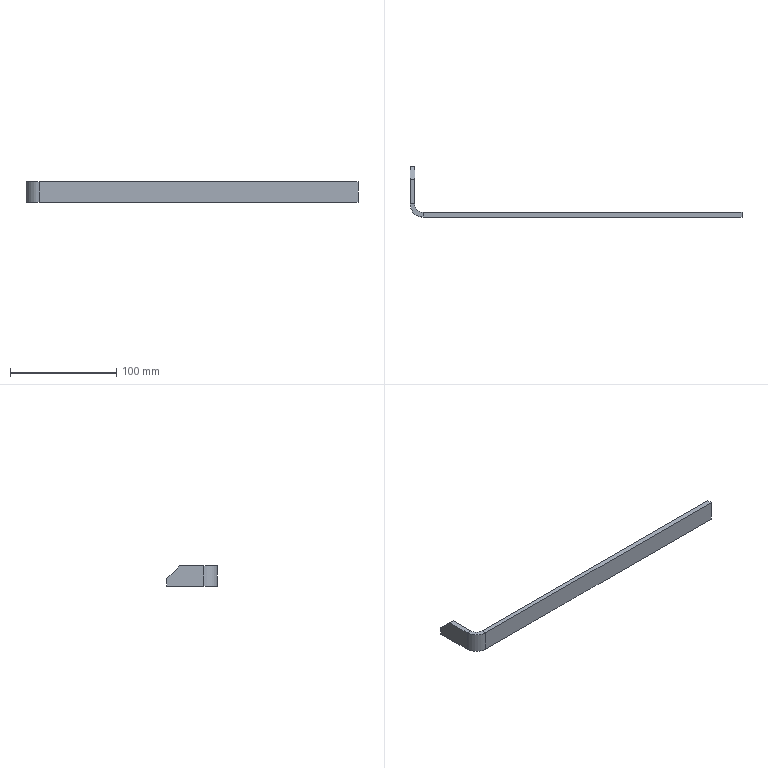Part | SolidWorks | features Chamfer 1, FlatPattern 1, SMBaseFlange 1, SheetMetal 1 | 1 solid | 15 faces | box 313 x 47.5 x 19 mm | volume 29738 mm3 | plane 13 | cylinder 2 | commonest cylinder face diameters 16 x1 25 x1
STEP:
#1=CARTESIAN_POINT('',(0.,-35.,9.5));
#2=VERTEX_POINT('',#1);
#3=CARTESIAN_POINT('',(4.5,-35.,9.5));
#4=VERTEX_POINT('',#3);
#5=CARTESIAN_POINT('',(0.,-35.,9.5));
#6=DIRECTION('',(1.,0.,0.));
#7=VECTOR('',#6,1000.);
#8=LINE('',#5,#7);
#9=EDGE_CURVE('',#2,#4,#8,.T.);
#10=ORIENTED_EDGE('',*,*,#9,.F.);
#11=CARTESIAN_POINT('',(12.5,-47.5,9.5));
#12=VERTEX_POINT('',#11);
#13=CARTESIAN_POINT('',(12.5,-35.,9.5));
#14=DIRECTION('',(0.,0.,1.));
#15=DIRECTION('',(-1.,0.,0.));
#16=AXIS2_PLACEMENT_3D('',#13,#14,#15);
#17=CIRCLE('',#16,12.5);
#18=EDGE_CURVE('',#2,#12,#17,.T.);
#19=ORIENTED_EDGE('',*,*,#18,.T.);
#20=CARTESIAN_POINT('',(12.5,-43.,9.5));
#21=VERTEX_POINT('',#20);
#22=CARTESIAN_POINT('',(12.5,-43.,9.5));
#23=DIRECTION('',(0.,-1.,0.));
#24=VECTOR('',#23,1000.);
#25=LINE('',#22,#24);
#26=EDGE_CURVE('',#21,#12,#25,.T.);
#27=ORIENTED_EDGE('',*,*,#26,.F.);
#28=CARTESIAN_POINT('',(12.5,-35.,9.5));
#29=DIRECTION('',(0.,0.,1.));
#30=DIRECTION('',(1.,0.,0.));
#31=AXIS2_PLACEMENT_3D('',#28,#29,#30);
#32=CIRCLE('',#31,8.);
#33=EDGE_CURVE('',#4,#21,#32,.T.);
#34=ORIENTED_EDGE('',*,*,#33,.F.);
#35=EDGE_LOOP('',(#10,#19,#27,#34));
#36=FACE_OUTER_BOUND('',#35,.T.);
#37=CARTESIAN_POINT('',(0.,-35.,9.5));
#38=DIRECTION('',(0.,0.,1.));
#39=DIRECTION('',(1.,0.,0.));
#40=AXIS2_PLACEMENT_3D('',#37,#38,#39);
#41=PLANE('',#40);
#42=ADVANCED_FACE('',(#36),#41,.T.);
#43=CARTESIAN_POINT('',(4.5,-12.,9.5));
#44=VERTEX_POINT('',#43);
#45=CARTESIAN_POINT('',(4.5,0.,9.5));
#46=DIRECTION('',(0.,-1.,0.));
#47=VECTOR('',#46,1000.);
#48=LINE('',#45,#47);
#49=EDGE_CURVE('',#44,#4,#48,.T.);
#50=ORIENTED_EDGE('',*,*,#49,.F.);
#51=CARTESIAN_POINT('',(0.,-12.,9.5));
#52=VERTEX_POINT('',#51);
#53=CARTESIAN_POINT('',(12.5,-12.,9.5));
#54=DIRECTION('',(-1.,0.,0.));
#55=VECTOR('',#54,1000.);
#56=LINE('',#53,#55);
#57=EDGE_CURVE('',#44,#52,#56,.T.);
#58=ORIENTED_EDGE('',*,*,#57,.T.);
#59=CARTESIAN_POINT('',(0.,0.,9.5));
#60=DIRECTION('',(0.,-1.,0.));
#61=VECTOR('',#60,1000.);
#62=LINE('',#59,#61);
#63=EDGE_CURVE('',#52,#2,#62,.T.);
#64=ORIENTED_EDGE('',*,*,#63,.T.);
#65=ORIENTED_EDGE('',*,*,#9,.T.);
#66=EDGE_LOOP('',(#50,#58,#64,#65));
#67=FACE_OUTER_BOUND('',#66,.T.);
#68=CARTESIAN_POINT('',(12.5,-43.,9.5));
#69=DIRECTION('',(0.,0.,1.));
#70=DIRECTION('',(1.,0.,0.));
#71=AXIS2_PLACEMENT_3D('',#68,#69,#70);
#72=PLANE('',#71);
#73=ADVANCED_FACE('',(#67),#72,.T.);
#74=CARTESIAN_POINT('',(12.5,-47.5,-9.5));
#75=VERTEX_POINT('',#74);
#76=CARTESIAN_POINT('',(12.5,-43.,-9.5));
#77=VERTEX_POINT('',#76);
#78=CARTESIAN_POINT('',(12.5,-47.5,-9.5));
#79=DIRECTION('',(0.,1.,0.));
#80=VECTOR('',#79,1000.);
#81=LINE('',#78,#80);
#82=EDGE_CURVE('',#75,#77,#81,.T.);
#83=ORIENTED_EDGE('',*,*,#82,.F.);
#84=CARTESIAN_POINT('',(0.,-35.,-9.5));
#85=VERTEX_POINT('',#84);
#86=CARTESIAN_POINT('',(12.5,-35.,-9.5));
#87=DIRECTION('',(0.,0.,1.));
#88=DIRECTION('',(-1.,0.,0.));
#89=AXIS2_PLACEMENT_3D('',#86,#87,#88);
#90=CIRCLE('',#89,12.5);
#91=EDGE_CURVE('',#85,#75,#90,.T.);
#92=ORIENTED_EDGE('',*,*,#91,.F.);
#93=CARTESIAN_POINT('',(4.5,-35.,-9.5));
#94=VERTEX_POINT('',#93);
#95=CARTESIAN_POINT('',(4.5,-35.,-9.5));
#96=DIRECTION('',(-1.,0.,0.));
#97=VECTOR('',#96,1000.);
#98=LINE('',#95,#97);
#99=EDGE_CURVE('',#94,#85,#98,.T.);
#100=ORIENTED_EDGE('',*,*,#99,.F.);
#101=CARTESIAN_POINT('',(12.5,-35.,-9.5));
#102=DIRECTION('',(0.,0.,1.));
#103=DIRECTION('',(1.,0.,0.));
#104=AXIS2_PLACEMENT_3D('',#101,#102,#103);
#105=CIRCLE('',#104,8.);
#106=EDGE_CURVE('',#94,#77,#105,.T.);
#107=ORIENTED_EDGE('',*,*,#106,.T.);
#108=EDGE_LOOP('',(#83,#92,#100,#107));
#109=FACE_OUTER_BOUND('',#108,.T.);
#110=CARTESIAN_POINT('',(12.5,-47.5,-9.5));
#111=DIRECTION('',(0.,0.,-1.));
#112=DIRECTION('',(-1.,0.,0.));
#113=AXIS2_PLACEMENT_3D('',#110,#111,#112);
#114=PLANE('',#113);
#115=ADVANCED_FACE('',(#109),#114,.T.);
#116=CARTESIAN_POINT('',(313.,-47.5,-9.5));
#117=VERTEX_POINT('',#116);
#118=CARTESIAN_POINT('',(0.,-47.5,-9.5));
#119=DIRECTION('',(1.,0.,0.));
#120=VECTOR('',#119,1000.);
#121=LINE('',#118,#120);
#122=EDGE_CURVE('',#75,#117,#121,.T.);
#123=ORIENTED_EDGE('',*,*,#122,.F.);
#124=ORIENTED_EDGE('',*,*,#82,.T.);
#125=CARTESIAN_POINT('',(313.,-43.,-9.5));
#126=VERTEX_POINT('',#125);
#127=CARTESIAN_POINT('',(0.,-43.,-9.5));
#128=DIRECTION('',(1.,0.,0.));
#129=VECTOR('',#128,1000.);
#130=LINE('',#127,#129);
#131=EDGE_CURVE('',#77,#126,#130,.T.);
#132=ORIENTED_EDGE('',*,*,#131,.T.);
#133=CARTESIAN_POINT('',(313.,-43.,-9.5));
#134=DIRECTION('',(0.,-1.,0.));
#135=VECTOR('',#134,1000.);
#136=LINE('',#133,#135);
#137=EDGE_CURVE('',#126,#117,#136,.T.);
#138=ORIENTED_EDGE('',*,*,#137,.T.);
#139=EDGE_LOOP('',(#123,#124,#132,#138));
#140=FACE_OUTER_BOUND('',#139,.T.);
#141=CARTESIAN_POINT('',(4.5,-35.,-9.5));
#142=DIRECTION('',(0.,0.,-1.));
#143=DIRECTION('',(-1.,0.,0.));
#144=AXIS2_PLACEMENT_3D('',#141,#142,#143);
#145=PLANE('',#144);
#146=ADVANCED_FACE('',(#140),#145,.T.);
#147=ORIENTED_EDGE('',*,*,#122,.T.);
#148=CARTESIAN_POINT('',(313.,-47.5,9.5));
#149=VERTEX_POINT('',#148);
#150=CARTESIAN_POINT('',(313.,-47.5,9.5));
#151=DIRECTION('',(0.,0.,-1.));
#152=VECTOR('',#151,1000.);
#153=LINE('',#150,#152);
#154=EDGE_CURVE('',#149,#117,#153,.T.);
#155=ORIENTED_EDGE('',*,*,#154,.F.);
#156=CARTESIAN_POINT('',(0.,-47.5,9.5));
#157=DIRECTION('',(1.,0.,0.));
#158=VECTOR('',#157,1000.);
#159=LINE('',#156,#158);
#160=EDGE_CURVE('',#12,#149,#159,.T.);
#161=ORIENTED_EDGE('',*,*,#160,.F.);
#162=CARTESIAN_POINT('',(12.5,-47.5,9.5));
#163=DIRECTION('',(0.,0.,-1.));
#164=VECTOR('',#163,1000.);
#165=LINE('',#162,#164);
#166=EDGE_CURVE('',#12,#75,#165,.T.);
#167=ORIENTED_EDGE('',*,*,#166,.T.);
#168=EDGE_LOOP('',(#147,#155,#161,#167));
#169=FACE_OUTER_BOUND('',#168,.T.);
#170=CARTESIAN_POINT('',(0.,-47.5,9.5));
#171=DIRECTION('',(0.,1.,0.));
#172=DIRECTION('',(0.,0.,1.));
#173=AXIS2_PLACEMENT_3D('',#170,#171,#172);
#174=PLANE('',#173);
#175=ADVANCED_FACE('',(#169),#174,.F.);
#176=ORIENTED_EDGE('',*,*,#137,.F.);
#177=CARTESIAN_POINT('',(313.,-43.,9.5));
#178=VERTEX_POINT('',#177);
#179=CARTESIAN_POINT('',(313.,-43.,9.5));
#180=DIRECTION('',(0.,0.,-1.));
#181=VECTOR('',#180,1000.);
#182=LINE('',#179,#181);
#183=EDGE_CURVE('',#178,#126,#182,.T.);
#184=ORIENTED_EDGE('',*,*,#183,.F.);
#185=CARTESIAN_POINT('',(313.,-43.,9.5));
#186=DIRECTION('',(0.,-1.,0.));
#187=VECTOR('',#186,1000.);
#188=LINE('',#185,#187);
#189=EDGE_CURVE('',#178,#149,#188,.T.);
#190=ORIENTED_EDGE('',*,*,#189,.T.);
#191=ORIENTED_EDGE('',*,*,#154,.T.);
#192=EDGE_LOOP('',(#176,#184,#190,#191));
#193=FACE_OUTER_BOUND('',#192,.T.);
#194=CARTESIAN_POINT('',(313.,-43.,9.5));
#195=DIRECTION('',(1.,0.,0.));
#196=DIRECTION('',(0.,0.,-1.));
#197=AXIS2_PLACEMENT_3D('',#194,#195,#196);
#198=PLANE('',#197);
#199=ADVANCED_FACE('',(#193),#198,.T.);
#200=ORIENTED_EDGE('',*,*,#131,.F.);
#201=CARTESIAN_POINT('',(12.5,-43.,9.5));
#202=DIRECTION('',(0.,0.,-1.));
#203=VECTOR('',#202,1000.);
#204=LINE('',#201,#203);
#205=EDGE_CURVE('',#21,#77,#204,.T.);
#206=ORIENTED_EDGE('',*,*,#205,.F.);
#207=CARTESIAN_POINT('',(0.,-43.,9.5));
#208=DIRECTION('',(1.,0.,0.));
#209=VECTOR('',#208,1000.);
#210=LINE('',#207,#209);
#211=EDGE_CURVE('',#21,#178,#210,.T.);
#212=ORIENTED_EDGE('',*,*,#211,.T.);
#213=ORIENTED_EDGE('',*,*,#183,.T.);
#214=EDGE_LOOP('',(#200,#206,#212,#213));
#215=FACE_OUTER_BOUND('',#214,.T.);
#216=CARTESIAN_POINT('',(0.,-43.,9.5));
#217=DIRECTION('',(0.,1.,0.));
#218=DIRECTION('',(0.,0.,1.));
#219=AXIS2_PLACEMENT_3D('',#216,#217,#218);
#220=PLANE('',#219);
#221=ADVANCED_FACE('',(#215),#220,.T.);
#222=ORIENTED_EDGE('',*,*,#106,.F.);
#223=CARTESIAN_POINT('',(4.5,-35.,9.5));
#224=DIRECTION('',(0.,0.,-1.));
#225=VECTOR('',#224,1000.);
#226=LINE('',#223,#225);
#227=EDGE_CURVE('',#4,#94,#226,.T.);
#228=ORIENTED_EDGE('',*,*,#227,.F.);
#229=ORIENTED_EDGE('',*,*,#33,.T.);
#230=ORIENTED_EDGE('',*,*,#205,.T.);
#231=EDGE_LOOP('',(#222,#228,#229,#230));
#232=FACE_OUTER_BOUND('',#231,.T.);
#233=CARTESIAN_POINT('',(12.5,-35.,9.5));
#234=DIRECTION('',(0.,0.,-1.));
#235=DIRECTION('',(-1.,0.,0.));
#236=AXIS2_PLACEMENT_3D('',#233,#234,#235);
#237=CYLINDRICAL_SURFACE('',#236,8.);
#238=ADVANCED_FACE('',(#232),#237,.F.);
#239=CARTESIAN_POINT('',(4.5,0.,-2.5));
#240=VERTEX_POINT('',#239);
#241=CARTESIAN_POINT('',(4.5,0.,-9.5));
#242=VERTEX_POINT('',#241);
#243=CARTESIAN_POINT('',(4.5,0.,9.5));
#244=DIRECTION('',(0.,0.,-1.));
#245=VECTOR('',#244,1000.);
#246=LINE('',#243,#245);
#247=EDGE_CURVE('',#240,#242,#246,.T.);
#248=ORIENTED_EDGE('',*,*,#247,.F.);
#249=CARTESIAN_POINT('',(4.5,-6.,3.5));
#250=DIRECTION('',(0.,-0.7071,0.7071));
#251=VECTOR('',#250,1000.);
#252=LINE('',#249,#251);
#253=EDGE_CURVE('',#240,#44,#252,.T.);
#254=ORIENTED_EDGE('',*,*,#253,.T.);
#255=ORIENTED_EDGE('',*,*,#49,.T.);
#256=ORIENTED_EDGE('',*,*,#227,.T.);
#257=CARTESIAN_POINT('',(4.5,0.,-9.5));
#258=DIRECTION('',(0.,-1.,0.));
#259=VECTOR('',#258,1000.);
#260=LINE('',#257,#259);
#261=EDGE_CURVE('',#242,#94,#260,.T.);
#262=ORIENTED_EDGE('',*,*,#261,.F.);
#263=EDGE_LOOP('',(#248,#254,#255,#256,#262));
#264=FACE_OUTER_BOUND('',#263,.T.);
#265=CARTESIAN_POINT('',(4.5,0.,9.5));
#266=DIRECTION('',(1.,0.,0.));
#267=DIRECTION('',(0.,1.,0.));
#268=AXIS2_PLACEMENT_3D('',#265,#266,#267);
#269=PLANE('',#268);
#270=ADVANCED_FACE('',(#264),#269,.T.);
#271=CARTESIAN_POINT('',(0.,0.,-2.5));
#272=VERTEX_POINT('',#271);
#273=CARTESIAN_POINT('',(0.,0.,-9.5));
#274=VERTEX_POINT('',#273);
#275=CARTESIAN_POINT('',(0.,0.,9.5));
#276=DIRECTION('',(0.,0.,-1.));
#277=VECTOR('',#276,1000.);
#278=LINE('',#275,#277);
#279=EDGE_CURVE('',#272,#274,#278,.T.);
#280=ORIENTED_EDGE('',*,*,#279,.F.);
#281=CARTESIAN_POINT('',(0.,0.,-2.5));
#282=DIRECTION('',(1.,0.,0.));
#283=VECTOR('',#282,1000.);
#284=LINE('',#281,#283);
#285=EDGE_CURVE('',#272,#240,#284,.T.);
#286=ORIENTED_EDGE('',*,*,#285,.T.);
#287=ORIENTED_EDGE('',*,*,#247,.T.);
#288=CARTESIAN_POINT('',(0.,0.,-9.5));
#289=DIRECTION('',(1.,0.,0.));
#290=VECTOR('',#289,1000.);
#291=LINE('',#288,#290);
#292=EDGE_CURVE('',#274,#242,#291,.T.);
#293=ORIENTED_EDGE('',*,*,#292,.F.);
#294=EDGE_LOOP('',(#280,#286,#287,#293));
#295=FACE_OUTER_BOUND('',#294,.T.);
#296=CARTESIAN_POINT('',(0.,0.,9.5));
#297=DIRECTION('',(0.,1.,0.));
#298=DIRECTION('',(-1.,0.,0.));
#299=AXIS2_PLACEMENT_3D('',#296,#297,#298);
#300=PLANE('',#299);
#301=ADVANCED_FACE('',(#295),#300,.T.);
#302=ORIENTED_EDGE('',*,*,#63,.F.);
#303=CARTESIAN_POINT('',(0.,0.,-2.5));
#304=DIRECTION('',(0.,0.7071,-0.7071));
#305=VECTOR('',#304,1000.);
#306=LINE('',#303,#305);
#307=EDGE_CURVE('',#52,#272,#306,.T.);
#308=ORIENTED_EDGE('',*,*,#307,.T.);
#309=ORIENTED_EDGE('',*,*,#279,.T.);
#310=CARTESIAN_POINT('',(0.,0.,-9.5));
#311=DIRECTION('',(0.,-1.,0.));
#312=VECTOR('',#311,1000.);
#313=LINE('',#310,#312);
#314=EDGE_CURVE('',#274,#85,#313,.T.);
#315=ORIENTED_EDGE('',*,*,#314,.T.);
#316=CARTESIAN_POINT('',(0.,-35.,9.5));
#317=DIRECTION('',(0.,0.,-1.));
#318=VECTOR('',#317,1000.);
#319=LINE('',#316,#318);
#320=EDGE_CURVE('',#2,#85,#319,.T.);
#321=ORIENTED_EDGE('',*,*,#320,.F.);
#322=EDGE_LOOP('',(#302,#308,#309,#315,#321));
#323=FACE_OUTER_BOUND('',#322,.T.);
#324=CARTESIAN_POINT('',(0.,0.,9.5));
#325=DIRECTION('',(1.,0.,0.));
#326=DIRECTION('',(0.,1.,0.));
#327=AXIS2_PLACEMENT_3D('',#324,#325,#326);
#328=PLANE('',#327);
#329=ADVANCED_FACE('',(#323),#328,.F.);
#330=ORIENTED_EDGE('',*,*,#91,.T.);
#331=ORIENTED_EDGE('',*,*,#166,.F.);
#332=ORIENTED_EDGE('',*,*,#18,.F.);
#333=ORIENTED_EDGE('',*,*,#320,.T.);
#334=EDGE_LOOP('',(#330,#331,#332,#333));
#335=FACE_OUTER_BOUND('',#334,.T.);
#336=CARTESIAN_POINT('',(12.5,-35.,9.5));
#337=DIRECTION('',(0.,0.,-1.));
#338=DIRECTION('',(-1.,0.,0.));
#339=AXIS2_PLACEMENT_3D('',#336,#337,#338);
#340=CYLINDRICAL_SURFACE('',#339,12.5);
#341=ADVANCED_FACE('',(#335),#340,.T.);
#342=ORIENTED_EDGE('',*,*,#160,.T.);
#343=ORIENTED_EDGE('',*,*,#189,.F.);
#344=ORIENTED_EDGE('',*,*,#211,.F.);
#345=ORIENTED_EDGE('',*,*,#26,.T.);
#346=EDGE_LOOP('',(#342,#343,#344,#345));
#347=FACE_OUTER_BOUND('',#346,.T.);
#348=CARTESIAN_POINT('',(12.5,-35.,9.5));
#349=DIRECTION('',(0.,0.,1.));
#350=DIRECTION('',(1.,0.,0.));
#351=AXIS2_PLACEMENT_3D('',#348,#349,#350);
#352=PLANE('',#351);
#353=ADVANCED_FACE('',(#347),#352,.T.);
#354=ORIENTED_EDGE('',*,*,#261,.T.);
#355=ORIENTED_EDGE('',*,*,#99,.T.);
#356=ORIENTED_EDGE('',*,*,#314,.F.);
#357=ORIENTED_EDGE('',*,*,#292,.T.);
#358=EDGE_LOOP('',(#354,#355,#356,#357));
#359=FACE_OUTER_BOUND('',#358,.T.);
#360=CARTESIAN_POINT('',(12.5,-35.,-9.5));
#361=DIRECTION('',(0.,0.,1.));
#362=DIRECTION('',(1.,0.,0.));
#363=AXIS2_PLACEMENT_3D('',#360,#361,#362);
#364=PLANE('',#363);
#365=ADVANCED_FACE('',(#359),#364,.F.);
#366=ORIENTED_EDGE('',*,*,#307,.F.);
#367=ORIENTED_EDGE('',*,*,#57,.F.);
#368=ORIENTED_EDGE('',*,*,#253,.F.);
#369=ORIENTED_EDGE('',*,*,#285,.F.);
#370=EDGE_LOOP('',(#366,#367,#368,#369));
#371=FACE_OUTER_BOUND('',#370,.T.);
#372=CARTESIAN_POINT('',(0.,0.,-2.5));
#373=DIRECTION('',(0.,-0.7071,-0.7071));
#374=DIRECTION('',(1.,0.,0.));
#375=AXIS2_PLACEMENT_3D('',#372,#373,#374);
#376=PLANE('',#375);
#377=ADVANCED_FACE('',(#371),#376,.F.);
#378=CLOSED_SHELL('',(#42,#73,#115,#146,#175,#199,#221,#238,#270,#301,#329,#341,#353,#365,#377));
#379=MANIFOLD_SOLID_BREP('',#378);
#380=CARTESIAN_POINT('',(0.,0.,0.));
#381=DIRECTION('',(0.,0.,1.));
#382=DIRECTION('',(1.,0.,0.));
#383=AXIS2_PLACEMENT_3D('',#380,#381,#382);
#384=(LENGTH_UNIT()NAMED_UNIT(*)SI_UNIT(.MILLI.,.METRE.));
#385=UNCERTAINTY_MEASURE_WITH_UNIT(LENGTH_MEASURE(0.00001),#384,'','');
#386=(NAMED_UNIT(*)PLANE_ANGLE_UNIT()SI_UNIT($,.RADIAN.));
#387=(NAMED_UNIT(*)SI_UNIT($,.STERADIAN.)SOLID_ANGLE_UNIT());
#388=(GEOMETRIC_REPRESENTATION_CONTEXT(3)GLOBAL_UNCERTAINTY_ASSIGNED_CONTEXT((#385))GLOBAL_UNIT_ASSIGNED_CONTEXT((#384,#386,#387))REPRESENTATION_CONTEXT('',''));
#389=ADVANCED_BREP_SHAPE_REPRESENTATION('',(#379,#383),#388);